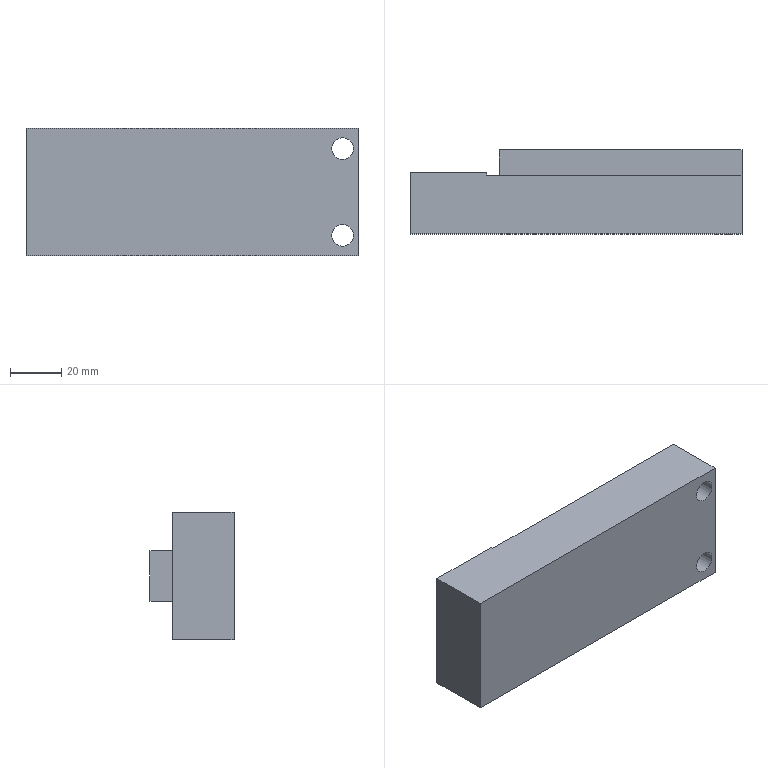Part | STEP file | SHIM SUPPORT | 1 solid | 18 faces | box 130 x 32.9 x 50 mm | volume 166423 mm3 | plane 12 | cylinder 4 | cone 2 | commonest cylinder face diameters 4.917 x2 8.5 x2
STEP:
#1=CARTESIAN_POINT('',(0.,0.,0.));
#2=DIRECTION('',(0.,0.,1.));
#3=DIRECTION('',(1.,0.,0.));
#4=AXIS2_PLACEMENT_3D('',#1,#2,#3);
#5=CARTESIAN_POINT('',(-103.5,89.682,-15.1));
#6=VERTEX_POINT('',#5);
#7=CARTESIAN_POINT('',(-103.5,79.782,-15.1));
#8=VERTEX_POINT('',#7);
#9=CARTESIAN_POINT('',(-103.5,89.682,-15.1));
#10=DIRECTION('',(0.,-1.,0.));
#11=VECTOR('',#10,1.);
#12=LINE('',#9,#11);
#13=CARTESIAN_POINT('',(-103.5,89.682,-34.9));
#14=DIRECTION('',(1.,0.,0.));
#15=DIRECTION('',(0.,0.,-1.));
#16=AXIS2_PLACEMENT_3D('',#13,#14,#15);
#17=PLANE('',#16);
#18=CARTESIAN_POINT('',(-19.8,0.));
#19=DIRECTION('',(0.,-1.));
#20=VECTOR('',#19,1.);
#21=LINE('',#18,#20);
#22=(GEOMETRIC_REPRESENTATION_CONTEXT(2)PARAMETRIC_REPRESENTATION_CONTEXT()REPRESENTATION_CONTEXT('',''));
#23=DEFINITIONAL_REPRESENTATION('',(#21),#22);
#24=PCURVE('',#17,#23);
#25=CARTESIAN_POINT('',(-108.5,79.782,-15.1));
#26=DIRECTION('',(0.,0.,1.));
#27=DIRECTION('',(1.,0.,0.));
#28=AXIS2_PLACEMENT_3D('',#25,#26,#27);
#29=PLANE('',#28);
#30=CARTESIAN_POINT('',(5.,9.9));
#31=DIRECTION('',(0.,-1.));
#32=VECTOR('',#31,1.);
#33=LINE('',#30,#32);
#34=(GEOMETRIC_REPRESENTATION_CONTEXT(2)PARAMETRIC_REPRESENTATION_CONTEXT()REPRESENTATION_CONTEXT('',''));
#35=DEFINITIONAL_REPRESENTATION('',(#33),#34);
#36=PCURVE('',#29,#35);
#37=SURFACE_CURVE('',#12,(#24,#36),.PCURVE_S1.);
#38=EDGE_CURVE('',#6,#8,#37,.T.);
#39=ORIENTED_EDGE('',*,*,#38,.F.);
#40=CARTESIAN_POINT('',(-103.5,89.682,-34.9));
#41=VERTEX_POINT('',#40);
#42=CARTESIAN_POINT('',(-103.5,89.682,-34.9));
#43=DIRECTION('',(0.,0.,1.));
#44=VECTOR('',#43,1.);
#45=LINE('',#42,#44);
#46=CARTESIAN_POINT('',(0.,0.));
#47=DIRECTION('',(-1.,0.));
#48=VECTOR('',#47,1.);
#49=LINE('',#46,#48);
#50=(GEOMETRIC_REPRESENTATION_CONTEXT(2)PARAMETRIC_REPRESENTATION_CONTEXT()REPRESENTATION_CONTEXT('',''));
#51=DEFINITIONAL_REPRESENTATION('',(#49),#50);
#52=PCURVE('',#17,#51);
#53=CARTESIAN_POINT('',(-108.5,89.682,-15.1));
#54=DIRECTION('',(0.,1.,0.));
#55=DIRECTION('',(0.,0.,1.));
#56=AXIS2_PLACEMENT_3D('',#53,#54,#55);
#57=PLANE('',#56);
#58=CARTESIAN_POINT('',(-19.8,5.));
#59=DIRECTION('',(1.,0.));
#60=VECTOR('',#59,1.);
#61=LINE('',#58,#60);
#62=(GEOMETRIC_REPRESENTATION_CONTEXT(2)PARAMETRIC_REPRESENTATION_CONTEXT()REPRESENTATION_CONTEXT('',''));
#63=DEFINITIONAL_REPRESENTATION('',(#61),#62);
#64=PCURVE('',#57,#63);
#65=SURFACE_CURVE('',#45,(#52,#64),.PCURVE_S1.);
#66=EDGE_CURVE('',#41,#6,#65,.T.);
#67=ORIENTED_EDGE('',*,*,#66,.F.);
#68=CARTESIAN_POINT('',(-103.5,79.782,-34.9));
#69=VERTEX_POINT('',#68);
#70=CARTESIAN_POINT('',(-103.5,79.782,-34.9));
#71=DIRECTION('',(0.,1.,0.));
#72=VECTOR('',#71,1.);
#73=LINE('',#70,#72);
#74=CARTESIAN_POINT('',(0.,-9.9));
#75=DIRECTION('',(0.,1.));
#76=VECTOR('',#75,1.);
#77=LINE('',#74,#76);
#78=(GEOMETRIC_REPRESENTATION_CONTEXT(2)PARAMETRIC_REPRESENTATION_CONTEXT()REPRESENTATION_CONTEXT('',''));
#79=DEFINITIONAL_REPRESENTATION('',(#77),#78);
#80=PCURVE('',#17,#79);
#81=CARTESIAN_POINT('',(-108.5,89.682,-34.9));
#82=DIRECTION('',(0.,0.,-1.));
#83=DIRECTION('',(-1.,0.,0.));
#84=AXIS2_PLACEMENT_3D('',#81,#82,#83);
#85=PLANE('',#84);
#86=CARTESIAN_POINT('',(-5.,-9.9));
#87=DIRECTION('',(0.,1.));
#88=VECTOR('',#87,1.);
#89=LINE('',#86,#88);
#90=(GEOMETRIC_REPRESENTATION_CONTEXT(2)PARAMETRIC_REPRESENTATION_CONTEXT()REPRESENTATION_CONTEXT('',''));
#91=DEFINITIONAL_REPRESENTATION('',(#89),#90);
#92=PCURVE('',#85,#91);
#93=SURFACE_CURVE('',#73,(#80,#92),.PCURVE_S1.);
#94=EDGE_CURVE('',#69,#41,#93,.T.);
#95=ORIENTED_EDGE('',*,*,#94,.F.);
#96=CARTESIAN_POINT('',(-103.5,79.782,-34.9));
#97=DIRECTION('',(0.,0.,1.));
#98=VECTOR('',#97,1.);
#99=LINE('',#96,#98);
#100=CARTESIAN_POINT('',(0.,-9.9));
#101=DIRECTION('',(-1.,0.));
#102=VECTOR('',#101,1.);
#103=LINE('',#100,#102);
#104=(GEOMETRIC_REPRESENTATION_CONTEXT(2)PARAMETRIC_REPRESENTATION_CONTEXT()REPRESENTATION_CONTEXT('',''));
#105=DEFINITIONAL_REPRESENTATION('',(#103),#104);
#106=PCURVE('',#17,#105);
#107=CARTESIAN_POINT('',(-8.5,79.782,0.));
#108=DIRECTION('',(0.,1.,0.));
#109=DIRECTION('',(0.,0.,1.));
#110=AXIS2_PLACEMENT_3D('',#107,#108,#109);
#111=PLANE('',#110);
#112=CARTESIAN_POINT('',(-34.9,-95.));
#113=DIRECTION('',(1.,0.));
#114=VECTOR('',#113,1.);
#115=LINE('',#112,#114);
#116=(GEOMETRIC_REPRESENTATION_CONTEXT(2)PARAMETRIC_REPRESENTATION_CONTEXT()REPRESENTATION_CONTEXT('',''));
#117=DEFINITIONAL_REPRESENTATION('',(#115),#116);
#118=PCURVE('',#111,#117);
#119=SURFACE_CURVE('',#99,(#106,#118),.PCURVE_S1.);
#120=EDGE_CURVE('',#69,#8,#119,.T.);
#121=ORIENTED_EDGE('',*,*,#120,.T.);
#122=EDGE_LOOP('',(#39,#67,#95,#121));
#123=FACE_BOUND('',#122,.T.);
#124=ADVANCED_FACE('',(#123),#17,.F.);
#125=ORIENTED_EDGE('',*,*,#94,.T.);
#126=CARTESIAN_POINT('',(-8.5,89.682,-34.9));
#127=VERTEX_POINT('',#126);
#128=CARTESIAN_POINT('',(-103.5,89.682,-34.9));
#129=DIRECTION('',(1.,0.,0.));
#130=VECTOR('',#129,1.);
#131=LINE('',#128,#130);
#132=CARTESIAN_POINT('',(-5.,0.));
#133=DIRECTION('',(-1.,0.));
#134=VECTOR('',#133,1.);
#135=LINE('',#132,#134);
#136=(GEOMETRIC_REPRESENTATION_CONTEXT(2)PARAMETRIC_REPRESENTATION_CONTEXT()REPRESENTATION_CONTEXT('',''));
#137=DEFINITIONAL_REPRESENTATION('',(#135),#136);
#138=PCURVE('',#85,#137);
#139=CARTESIAN_POINT('',(-19.8,5.));
#140=DIRECTION('',(0.,1.));
#141=VECTOR('',#140,1.);
#142=LINE('',#139,#141);
#143=(GEOMETRIC_REPRESENTATION_CONTEXT(2)PARAMETRIC_REPRESENTATION_CONTEXT()REPRESENTATION_CONTEXT('',''));
#144=DEFINITIONAL_REPRESENTATION('',(#142),#143);
#145=PCURVE('',#57,#144);
#146=SURFACE_CURVE('',#131,(#138,#145),.PCURVE_S1.);
#147=EDGE_CURVE('',#41,#127,#146,.T.);
#148=ORIENTED_EDGE('',*,*,#147,.T.);
#149=CARTESIAN_POINT('',(-8.5,79.782,-34.9));
#150=VERTEX_POINT('',#149);
#151=CARTESIAN_POINT('',(-8.5,89.682,-34.9));
#152=DIRECTION('',(0.,-1.,0.));
#153=VECTOR('',#152,1.);
#154=LINE('',#151,#153);
#155=CARTESIAN_POINT('',(-100.,0.));
#156=DIRECTION('',(0.,-1.));
#157=VECTOR('',#156,1.);
#158=LINE('',#155,#157);
#159=(GEOMETRIC_REPRESENTATION_CONTEXT(2)PARAMETRIC_REPRESENTATION_CONTEXT()REPRESENTATION_CONTEXT('',''));
#160=DEFINITIONAL_REPRESENTATION('',(#158),#159);
#161=PCURVE('',#85,#160);
#162=CARTESIAN_POINT('',(-8.5,56.782,0.));
#163=DIRECTION('',(1.,0.,0.));
#164=DIRECTION('',(0.,0.,-1.));
#165=AXIS2_PLACEMENT_3D('',#162,#163,#164);
#166=PLANE('',#165);
#167=CARTESIAN_POINT('',(34.9,32.9));
#168=DIRECTION('',(0.,-1.));
#169=VECTOR('',#168,1.);
#170=LINE('',#167,#169);
#171=(GEOMETRIC_REPRESENTATION_CONTEXT(2)PARAMETRIC_REPRESENTATION_CONTEXT()REPRESENTATION_CONTEXT('',''));
#172=DEFINITIONAL_REPRESENTATION('',(#170),#171);
#173=PCURVE('',#166,#172);
#174=SURFACE_CURVE('',#154,(#161,#173),.PCURVE_S1.);
#175=EDGE_CURVE('',#127,#150,#174,.T.);
#176=ORIENTED_EDGE('',*,*,#175,.T.);
#177=CARTESIAN_POINT('',(-103.5,79.782,-34.9));
#178=DIRECTION('',(1.,0.,0.));
#179=VECTOR('',#178,1.);
#180=LINE('',#177,#179);
#181=CARTESIAN_POINT('',(-5.,-9.9));
#182=DIRECTION('',(-1.,0.));
#183=VECTOR('',#182,1.);
#184=LINE('',#181,#183);
#185=(GEOMETRIC_REPRESENTATION_CONTEXT(2)PARAMETRIC_REPRESENTATION_CONTEXT()REPRESENTATION_CONTEXT('',''));
#186=DEFINITIONAL_REPRESENTATION('',(#184),#185);
#187=PCURVE('',#85,#186);
#188=CARTESIAN_POINT('',(-34.9,-95.));
#189=DIRECTION('',(0.,1.));
#190=VECTOR('',#189,1.);
#191=LINE('',#188,#190);
#192=(GEOMETRIC_REPRESENTATION_CONTEXT(2)PARAMETRIC_REPRESENTATION_CONTEXT()REPRESENTATION_CONTEXT('',''));
#193=DEFINITIONAL_REPRESENTATION('',(#191),#192);
#194=PCURVE('',#111,#193);
#195=SURFACE_CURVE('',#180,(#187,#194),.PCURVE_S1.);
#196=EDGE_CURVE('',#69,#150,#195,.T.);
#197=ORIENTED_EDGE('',*,*,#196,.F.);
#198=EDGE_LOOP('',(#125,#148,#176,#197));
#199=FACE_BOUND('',#198,.T.);
#200=ADVANCED_FACE('',(#199),#85,.T.);
#201=ORIENTED_EDGE('',*,*,#66,.T.);
#202=CARTESIAN_POINT('',(-8.5,89.682,-15.1));
#203=VERTEX_POINT('',#202);
#204=CARTESIAN_POINT('',(-103.5,89.682,-15.1));
#205=DIRECTION('',(1.,0.,0.));
#206=VECTOR('',#205,1.);
#207=LINE('',#204,#206);
#208=CARTESIAN_POINT('',(0.,5.));
#209=DIRECTION('',(0.,1.));
#210=VECTOR('',#209,1.);
#211=LINE('',#208,#210);
#212=(GEOMETRIC_REPRESENTATION_CONTEXT(2)PARAMETRIC_REPRESENTATION_CONTEXT()REPRESENTATION_CONTEXT('',''));
#213=DEFINITIONAL_REPRESENTATION('',(#211),#212);
#214=PCURVE('',#57,#213);
#215=CARTESIAN_POINT('',(5.,9.9));
#216=DIRECTION('',(1.,0.));
#217=VECTOR('',#216,1.);
#218=LINE('',#215,#217);
#219=(GEOMETRIC_REPRESENTATION_CONTEXT(2)PARAMETRIC_REPRESENTATION_CONTEXT()REPRESENTATION_CONTEXT('',''));
#220=DEFINITIONAL_REPRESENTATION('',(#218),#219);
#221=PCURVE('',#29,#220);
#222=SURFACE_CURVE('',#207,(#214,#221),.PCURVE_S1.);
#223=EDGE_CURVE('',#6,#203,#222,.T.);
#224=ORIENTED_EDGE('',*,*,#223,.T.);
#225=CARTESIAN_POINT('',(-8.5,89.682,-15.1));
#226=DIRECTION('',(0.,0.,-1.));
#227=VECTOR('',#226,1.);
#228=LINE('',#225,#227);
#229=CARTESIAN_POINT('',(0.,100.));
#230=DIRECTION('',(-1.,0.));
#231=VECTOR('',#230,1.);
#232=LINE('',#229,#231);
#233=(GEOMETRIC_REPRESENTATION_CONTEXT(2)PARAMETRIC_REPRESENTATION_CONTEXT()REPRESENTATION_CONTEXT('',''));
#234=DEFINITIONAL_REPRESENTATION('',(#232),#233);
#235=PCURVE('',#57,#234);
#236=CARTESIAN_POINT('',(15.1,32.9));
#237=DIRECTION('',(1.,0.));
#238=VECTOR('',#237,1.);
#239=LINE('',#236,#238);
#240=(GEOMETRIC_REPRESENTATION_CONTEXT(2)PARAMETRIC_REPRESENTATION_CONTEXT()REPRESENTATION_CONTEXT('',''));
#241=DEFINITIONAL_REPRESENTATION('',(#239),#240);
#242=PCURVE('',#166,#241);
#243=SURFACE_CURVE('',#228,(#235,#242),.PCURVE_S1.);
#244=EDGE_CURVE('',#203,#127,#243,.T.);
#245=ORIENTED_EDGE('',*,*,#244,.T.);
#246=ORIENTED_EDGE('',*,*,#147,.F.);
#247=EDGE_LOOP('',(#201,#224,#245,#246));
#248=FACE_BOUND('',#247,.T.);
#249=ADVANCED_FACE('',(#248),#57,.T.);
#250=CARTESIAN_POINT('',(-114.775,65.782,-5.));
#251=VERTEX_POINT('',#250);
#252=CARTESIAN_POINT('',(-117.233,65.782,-5.));
#253=DIRECTION('',(0.,1.,0.));
#254=DIRECTION('',(1.,0.,0.));
#255=AXIS2_PLACEMENT_3D('',#252,#253,#254);
#256=CIRCLE('',#255,2.458);
#257=CARTESIAN_POINT('',(-117.233,65.043,-5.));
#258=DIRECTION('',(0.,1.,0.));
#259=DIRECTION('',(1.,0.,0.));
#260=AXIS2_PLACEMENT_3D('',#257,#258,#259);
#261=CONICAL_SURFACE('',#260,1.229,1.03);
#262=CARTESIAN_POINT('',(0.,0.7386));
#263=DIRECTION('',(1.,0.));
#264=VECTOR('',#263,1.);
#265=LINE('',#262,#264);
#266=(GEOMETRIC_REPRESENTATION_CONTEXT(2)PARAMETRIC_REPRESENTATION_CONTEXT()REPRESENTATION_CONTEXT('',''));
#267=DEFINITIONAL_REPRESENTATION('',(#265),#266);
#268=PCURVE('',#261,#267);
#269=CARTESIAN_POINT('',(-117.233,73.282,-5.));
#270=DIRECTION('',(0.,1.,0.));
#271=DIRECTION('',(1.,0.,0.));
#272=AXIS2_PLACEMENT_3D('',#269,#270,#271);
#273=CYLINDRICAL_SURFACE('',#272,2.458);
#274=CARTESIAN_POINT('',(0.,-7.5));
#275=DIRECTION('',(1.,0.));
#276=VECTOR('',#275,1.);
#277=LINE('',#274,#276);
#278=(GEOMETRIC_REPRESENTATION_CONTEXT(2)PARAMETRIC_REPRESENTATION_CONTEXT()REPRESENTATION_CONTEXT('',''));
#279=DEFINITIONAL_REPRESENTATION('',(#277),#278);
#280=PCURVE('',#273,#279);
#281=SURFACE_CURVE('',#256,(#268,#280),.PCURVE_S1.);
#282=EDGE_CURVE('',#251,#251,#281,.T.);
#283=ORIENTED_EDGE('',*,*,#282,.F.);
#284=CARTESIAN_POINT('',(-117.233,64.304,-5.));
#285=VERTEX_POINT('',#284);
#286=CARTESIAN_POINT('',(-117.233,64.304,-5.));
#287=CARTESIAN_POINT('',(-114.775,65.782,-5.));
#288=B_SPLINE_CURVE_WITH_KNOTS('',1,(#286,#287),.UNSPECIFIED.,.F.,.F.,(2,2),(-1.434,1.434),.PIECEWISE_BEZIER_KNOTS.);
#289=CARTESIAN_POINT('',(0.,0.));
#290=DIRECTION('',(0.,1.));
#291=VECTOR('',#290,1.);
#292=LINE('',#289,#291);
#293=(GEOMETRIC_REPRESENTATION_CONTEXT(2)PARAMETRIC_REPRESENTATION_CONTEXT()REPRESENTATION_CONTEXT('',''));
#294=DEFINITIONAL_REPRESENTATION('',(#292),#293);
#295=PCURVE('',#261,#294);
#296=CARTESIAN_POINT('',(6.283,0.));
#297=DIRECTION('',(0.,1.));
#298=VECTOR('',#297,1.);
#299=LINE('',#296,#298);
#300=(GEOMETRIC_REPRESENTATION_CONTEXT(2)PARAMETRIC_REPRESENTATION_CONTEXT()REPRESENTATION_CONTEXT('',''));
#301=DEFINITIONAL_REPRESENTATION('',(#299),#300);
#302=PCURVE('',#261,#301);
#303=SEAM_CURVE('',#288,(#295,#302),.PCURVE_S1.);
#304=EDGE_CURVE('',#285,#251,#303,.T.);
#305=ORIENTED_EDGE('',*,*,#304,.F.);
#306=ORIENTED_EDGE('',*,*,#304,.T.);
#307=EDGE_LOOP('',(#283,#305,#306));
#308=FACE_BOUND('',#307,.F.);
#309=ADVANCED_FACE('',(#308),#261,.F.);
#310=CARTESIAN_POINT('',(-114.775,80.782,-5.));
#311=VERTEX_POINT('',#310);
#312=CARTESIAN_POINT('',(-117.233,80.782,-5.));
#313=DIRECTION('',(0.,-1.,0.));
#314=DIRECTION('',(1.,0.,0.));
#315=AXIS2_PLACEMENT_3D('',#312,#313,#314);
#316=CIRCLE('',#315,2.458);
#317=CARTESIAN_POINT('',(6.283,7.5));
#318=DIRECTION('',(-1.,0.));
#319=VECTOR('',#318,1.);
#320=LINE('',#317,#319);
#321=(GEOMETRIC_REPRESENTATION_CONTEXT(2)PARAMETRIC_REPRESENTATION_CONTEXT()REPRESENTATION_CONTEXT('',''));
#322=DEFINITIONAL_REPRESENTATION('',(#320),#321);
#323=PCURVE('',#273,#322);
#324=CARTESIAN_POINT('',(-108.5,80.782,-50.));
#325=DIRECTION('',(0.,1.,0.));
#326=DIRECTION('',(0.,0.,1.));
#327=AXIS2_PLACEMENT_3D('',#324,#325,#326);
#328=PLANE('',#327);
#329=CARTESIAN_POINT('',(45.,-6.275));
#330=CARTESIAN_POINT('',(49.258,-6.275));
#331=CARTESIAN_POINT('',(47.129,-9.962));
#332=CARTESIAN_POINT('',(45.,-13.65));
#333=CARTESIAN_POINT('',(42.871,-9.962));
#334=CARTESIAN_POINT('',(40.742,-6.275));
#335=CARTESIAN_POINT('',(45.,-6.275));
#336=(BOUNDED_CURVE()B_SPLINE_CURVE(2,(#329,#330,#331,#332,#333,#334,#335),.UNSPECIFIED.,.T.,.F.)B_SPLINE_CURVE_WITH_KNOTS((1,2,2,2,2,1),(-2.094,0.,2.094,4.189,6.283,8.378),.UNSPECIFIED.)CURVE()GEOMETRIC_REPRESENTATION_ITEM()RATIONAL_B_SPLINE_CURVE((1.,0.5,1.,0.5,1.,0.5,1.))REPRESENTATION_ITEM(''));
#337=(GEOMETRIC_REPRESENTATION_CONTEXT(2)PARAMETRIC_REPRESENTATION_CONTEXT()REPRESENTATION_CONTEXT('',''));
#338=DEFINITIONAL_REPRESENTATION('',(#336),#337);
#339=PCURVE('',#328,#338);
#340=SURFACE_CURVE('',#316,(#323,#339),.PCURVE_S1.);
#341=EDGE_CURVE('',#311,#311,#340,.T.);
#342=ORIENTED_EDGE('',*,*,#341,.T.);
#343=CARTESIAN_POINT('',(-114.775,65.782,-5.));
#344=CARTESIAN_POINT('',(-114.775,80.782,-5.));
#345=B_SPLINE_CURVE_WITH_KNOTS('',1,(#343,#344),.UNSPECIFIED.,.F.,.F.,(2,2),(-7.5,7.5),.PIECEWISE_BEZIER_KNOTS.);
#346=CARTESIAN_POINT('',(0.,0.));
#347=DIRECTION('',(0.,1.));
#348=VECTOR('',#347,1.);
#349=LINE('',#346,#348);
#350=(GEOMETRIC_REPRESENTATION_CONTEXT(2)PARAMETRIC_REPRESENTATION_CONTEXT()REPRESENTATION_CONTEXT('',''));
#351=DEFINITIONAL_REPRESENTATION('',(#349),#350);
#352=PCURVE('',#273,#351);
#353=CARTESIAN_POINT('',(6.283,0.));
#354=DIRECTION('',(0.,1.));
#355=VECTOR('',#354,1.);
#356=LINE('',#353,#355);
#357=(GEOMETRIC_REPRESENTATION_CONTEXT(2)PARAMETRIC_REPRESENTATION_CONTEXT()REPRESENTATION_CONTEXT('',''));
#358=DEFINITIONAL_REPRESENTATION('',(#356),#357);
#359=PCURVE('',#273,#358);
#360=SEAM_CURVE('',#345,(#352,#359),.PCURVE_S1.);
#361=EDGE_CURVE('',#251,#311,#360,.T.);
#362=ORIENTED_EDGE('',*,*,#361,.F.);
#363=ORIENTED_EDGE('',*,*,#282,.T.);
#364=ORIENTED_EDGE('',*,*,#361,.T.);
#365=EDGE_LOOP('',(#342,#362,#363,#364));
#366=FACE_BOUND('',#365,.F.);
#367=ADVANCED_FACE('',(#366),#273,.F.);
#368=CARTESIAN_POINT('',(-114.775,65.782,-45.));
#369=VERTEX_POINT('',#368);
#370=CARTESIAN_POINT('',(-117.233,65.782,-45.));
#371=DIRECTION('',(0.,1.,0.));
#372=DIRECTION('',(1.,0.,0.));
#373=AXIS2_PLACEMENT_3D('',#370,#371,#372);
#374=CIRCLE('',#373,2.458);
#375=CARTESIAN_POINT('',(-117.233,65.043,-45.));
#376=DIRECTION('',(0.,1.,0.));
#377=DIRECTION('',(1.,0.,0.));
#378=AXIS2_PLACEMENT_3D('',#375,#376,#377);
#379=CONICAL_SURFACE('',#378,1.229,1.03);
#380=CARTESIAN_POINT('',(0.,0.7386));
#381=DIRECTION('',(1.,0.));
#382=VECTOR('',#381,1.);
#383=LINE('',#380,#382);
#384=(GEOMETRIC_REPRESENTATION_CONTEXT(2)PARAMETRIC_REPRESENTATION_CONTEXT()REPRESENTATION_CONTEXT('',''));
#385=DEFINITIONAL_REPRESENTATION('',(#383),#384);
#386=PCURVE('',#379,#385);
#387=CARTESIAN_POINT('',(-117.233,73.282,-45.));
#388=DIRECTION('',(0.,1.,0.));
#389=DIRECTION('',(1.,0.,0.));
#390=AXIS2_PLACEMENT_3D('',#387,#388,#389);
#391=CYLINDRICAL_SURFACE('',#390,2.458);
#392=CARTESIAN_POINT('',(0.,-7.5));
#393=DIRECTION('',(1.,0.));
#394=VECTOR('',#393,1.);
#395=LINE('',#392,#394);
#396=(GEOMETRIC_REPRESENTATION_CONTEXT(2)PARAMETRIC_REPRESENTATION_CONTEXT()REPRESENTATION_CONTEXT('',''));
#397=DEFINITIONAL_REPRESENTATION('',(#395),#396);
#398=PCURVE('',#391,#397);
#399=SURFACE_CURVE('',#374,(#386,#398),.PCURVE_S1.);
#400=EDGE_CURVE('',#369,#369,#399,.T.);
#401=ORIENTED_EDGE('',*,*,#400,.F.);
#402=CARTESIAN_POINT('',(-117.233,64.304,-45.));
#403=VERTEX_POINT('',#402);
#404=CARTESIAN_POINT('',(-117.233,64.304,-45.));
#405=CARTESIAN_POINT('',(-114.775,65.782,-45.));
#406=B_SPLINE_CURVE_WITH_KNOTS('',1,(#404,#405),.UNSPECIFIED.,.F.,.F.,(2,2),(-1.434,1.434),.PIECEWISE_BEZIER_KNOTS.);
#407=CARTESIAN_POINT('',(0.,0.));
#408=DIRECTION('',(0.,1.));
#409=VECTOR('',#408,1.);
#410=LINE('',#407,#409);
#411=(GEOMETRIC_REPRESENTATION_CONTEXT(2)PARAMETRIC_REPRESENTATION_CONTEXT()REPRESENTATION_CONTEXT('',''));
#412=DEFINITIONAL_REPRESENTATION('',(#410),#411);
#413=PCURVE('',#379,#412);
#414=CARTESIAN_POINT('',(6.283,0.));
#415=DIRECTION('',(0.,1.));
#416=VECTOR('',#415,1.);
#417=LINE('',#414,#416);
#418=(GEOMETRIC_REPRESENTATION_CONTEXT(2)PARAMETRIC_REPRESENTATION_CONTEXT()REPRESENTATION_CONTEXT('',''));
#419=DEFINITIONAL_REPRESENTATION('',(#417),#418);
#420=PCURVE('',#379,#419);
#421=SEAM_CURVE('',#406,(#413,#420),.PCURVE_S1.);
#422=EDGE_CURVE('',#403,#369,#421,.T.);
#423=ORIENTED_EDGE('',*,*,#422,.F.);
#424=ORIENTED_EDGE('',*,*,#422,.T.);
#425=EDGE_LOOP('',(#401,#423,#424));
#426=FACE_BOUND('',#425,.F.);
#427=ADVANCED_FACE('',(#426),#379,.F.);
#428=CARTESIAN_POINT('',(-114.775,80.782,-45.));
#429=VERTEX_POINT('',#428);
#430=CARTESIAN_POINT('',(-117.233,80.782,-45.));
#431=DIRECTION('',(0.,-1.,0.));
#432=DIRECTION('',(1.,0.,0.));
#433=AXIS2_PLACEMENT_3D('',#430,#431,#432);
#434=CIRCLE('',#433,2.458);
#435=CARTESIAN_POINT('',(6.283,7.5));
#436=DIRECTION('',(-1.,0.));
#437=VECTOR('',#436,1.);
#438=LINE('',#435,#437);
#439=(GEOMETRIC_REPRESENTATION_CONTEXT(2)PARAMETRIC_REPRESENTATION_CONTEXT()REPRESENTATION_CONTEXT('',''));
#440=DEFINITIONAL_REPRESENTATION('',(#438),#439);
#441=PCURVE('',#391,#440);
#442=CARTESIAN_POINT('',(5.,-6.275));
#443=CARTESIAN_POINT('',(9.258,-6.275));
#444=CARTESIAN_POINT('',(7.129,-9.962));
#445=CARTESIAN_POINT('',(5.,-13.65));
#446=CARTESIAN_POINT('',(2.871,-9.962));
#447=CARTESIAN_POINT('',(0.7418,-6.275));
#448=CARTESIAN_POINT('',(5.,-6.275));
#449=(BOUNDED_CURVE()B_SPLINE_CURVE(2,(#442,#443,#444,#445,#446,#447,#448),.UNSPECIFIED.,.T.,.F.)B_SPLINE_CURVE_WITH_KNOTS((1,2,2,2,2,1),(-2.094,0.,2.094,4.189,6.283,8.378),.UNSPECIFIED.)CURVE()GEOMETRIC_REPRESENTATION_ITEM()RATIONAL_B_SPLINE_CURVE((1.,0.5,1.,0.5,1.,0.5,1.))REPRESENTATION_ITEM(''));
#450=(GEOMETRIC_REPRESENTATION_CONTEXT(2)PARAMETRIC_REPRESENTATION_CONTEXT()REPRESENTATION_CONTEXT('',''));
#451=DEFINITIONAL_REPRESENTATION('',(#449),#450);
#452=PCURVE('',#328,#451);
#453=SURFACE_CURVE('',#434,(#441,#452),.PCURVE_S1.);
#454=EDGE_CURVE('',#429,#429,#453,.T.);
#455=ORIENTED_EDGE('',*,*,#454,.T.);
#456=CARTESIAN_POINT('',(-114.775,65.782,-45.));
#457=CARTESIAN_POINT('',(-114.775,80.782,-45.));
#458=B_SPLINE_CURVE_WITH_KNOTS('',1,(#456,#457),.UNSPECIFIED.,.F.,.F.,(2,2),(-7.5,7.5),.PIECEWISE_BEZIER_KNOTS.);
#459=CARTESIAN_POINT('',(0.,0.));
#460=DIRECTION('',(0.,1.));
#461=VECTOR('',#460,1.);
#462=LINE('',#459,#461);
#463=(GEOMETRIC_REPRESENTATION_CONTEXT(2)PARAMETRIC_REPRESENTATION_CONTEXT()REPRESENTATION_CONTEXT('',''));
#464=DEFINITIONAL_REPRESENTATION('',(#462),#463);
#465=PCURVE('',#391,#464);
#466=CARTESIAN_POINT('',(6.283,0.));
#467=DIRECTION('',(0.,1.));
#468=VECTOR('',#467,1.);
#469=LINE('',#466,#468);
#470=(GEOMETRIC_REPRESENTATION_CONTEXT(2)PARAMETRIC_REPRESENTATION_CONTEXT()REPRESENTATION_CONTEXT('',''));
#471=DEFINITIONAL_REPRESENTATION('',(#469),#470);
#472=PCURVE('',#391,#471);
#473=SEAM_CURVE('',#458,(#465,#472),.PCURVE_S1.);
#474=EDGE_CURVE('',#369,#429,#473,.T.);
#475=ORIENTED_EDGE('',*,*,#474,.F.);
#476=ORIENTED_EDGE('',*,*,#400,.T.);
#477=ORIENTED_EDGE('',*,*,#474,.T.);
#478=EDGE_LOOP('',(#455,#475,#476,#477));
#479=FACE_BOUND('',#478,.F.);
#480=ADVANCED_FACE('',(#479),#391,.F.);
#481=CARTESIAN_POINT('',(-18.75,56.782,-42.));
#482=VERTEX_POINT('',#481);
#483=CARTESIAN_POINT('',(-10.25,56.782,-42.));
#484=VERTEX_POINT('',#483);
#485=CARTESIAN_POINT('',(-14.5,56.782,-42.));
#486=DIRECTION('',(0.,1.,0.));
#487=DIRECTION('',(1.,0.,0.));
#488=AXIS2_PLACEMENT_3D('',#485,#486,#487);
#489=CIRCLE('',#488,4.25);
#490=CARTESIAN_POINT('',(-14.5,-63.335,-42.));
#491=DIRECTION('',(0.,1.,0.));
#492=DIRECTION('',(1.,0.,0.));
#493=AXIS2_PLACEMENT_3D('',#490,#491,#492);
#494=CYLINDRICAL_SURFACE('',#493,4.25);
#495=CARTESIAN_POINT('',(0.,120.117));
#496=DIRECTION('',(1.,0.));
#497=VECTOR('',#496,1.);
#498=LINE('',#495,#497);
#499=(GEOMETRIC_REPRESENTATION_CONTEXT(2)PARAMETRIC_REPRESENTATION_CONTEXT()REPRESENTATION_CONTEXT('',''));
#500=DEFINITIONAL_REPRESENTATION('',(#498),#499);
#501=PCURVE('',#494,#500);
#502=CARTESIAN_POINT('',(-18.5,56.782,0.));
#503=DIRECTION('',(0.,-1.,0.));
#504=DIRECTION('',(0.,0.,-1.));
#505=AXIS2_PLACEMENT_3D('',#502,#503,#504);
#506=PLANE('',#505);
#507=CARTESIAN_POINT('',(42.,8.25));
#508=CARTESIAN_POINT('',(49.361,8.25));
#509=CARTESIAN_POINT('',(45.681,1.875));
#510=CARTESIAN_POINT('',(42.,-4.5));
#511=CARTESIAN_POINT('',(38.319,1.875));
#512=CARTESIAN_POINT('',(34.639,8.25));
#513=CARTESIAN_POINT('',(42.,8.25));
#514=(BOUNDED_CURVE()B_SPLINE_CURVE(2,(#507,#508,#509,#510,#511,#512,#513),.UNSPECIFIED.,.T.,.F.)B_SPLINE_CURVE_WITH_KNOTS((1,2,2,2,2,1),(-2.094,0.,2.094,4.189,6.283,8.378),.UNSPECIFIED.)CURVE()GEOMETRIC_REPRESENTATION_ITEM()RATIONAL_B_SPLINE_CURVE((1.,0.5,1.,0.5,1.,0.5,1.))REPRESENTATION_ITEM(''));
#515=(GEOMETRIC_REPRESENTATION_CONTEXT(2)PARAMETRIC_REPRESENTATION_CONTEXT()REPRESENTATION_CONTEXT('',''));
#516=DEFINITIONAL_REPRESENTATION('',(#514),#515);
#517=PCURVE('',#506,#516);
#518=SURFACE_CURVE('',#489,(#501,#517),.PCURVE_S1.);
#519=EDGE_CURVE('',#482,#484,#518,.T.);
#520=ORIENTED_EDGE('',*,*,#519,.T.);
#521=CARTESIAN_POINT('',(-10.25,79.782,-42.));
#522=VERTEX_POINT('',#521);
#523=CARTESIAN_POINT('',(-10.25,56.782,-42.));
#524=CARTESIAN_POINT('',(-10.25,79.782,-42.));
#525=B_SPLINE_CURVE_WITH_KNOTS('',1,(#523,#524),.UNSPECIFIED.,.F.,.F.,(2,2),(120.117,143.117),.PIECEWISE_BEZIER_KNOTS.);
#526=CARTESIAN_POINT('',(6.283,0.));
#527=DIRECTION('',(0.,1.));
#528=VECTOR('',#527,1.);
#529=LINE('',#526,#528);
#530=(GEOMETRIC_REPRESENTATION_CONTEXT(2)PARAMETRIC_REPRESENTATION_CONTEXT()REPRESENTATION_CONTEXT('',''));
#531=DEFINITIONAL_REPRESENTATION('',(#529),#530);
#532=PCURVE('',#494,#531);
#533=CARTESIAN_POINT('',(0.,0.));
#534=DIRECTION('',(0.,1.));
#535=VECTOR('',#534,1.);
#536=LINE('',#533,#535);
#537=(GEOMETRIC_REPRESENTATION_CONTEXT(2)PARAMETRIC_REPRESENTATION_CONTEXT()REPRESENTATION_CONTEXT('',''));
#538=DEFINITIONAL_REPRESENTATION('',(#536),#537);
#539=PCURVE('',#494,#538);
#540=SEAM_CURVE('',#525,(#532,#539),.PCURVE_S1.);
#541=EDGE_CURVE('',#484,#522,#540,.T.);
#542=ORIENTED_EDGE('',*,*,#541,.T.);
#543=CARTESIAN_POINT('',(-14.5,79.782,-42.));
#544=DIRECTION('',(0.,-1.,0.));
#545=DIRECTION('',(1.,0.,0.));
#546=AXIS2_PLACEMENT_3D('',#543,#544,#545);
#547=CIRCLE('',#546,4.25);
#548=CARTESIAN_POINT('',(6.283,143.117));
#549=DIRECTION('',(-1.,0.));
#550=VECTOR('',#549,1.);
#551=LINE('',#548,#550);
#552=(GEOMETRIC_REPRESENTATION_CONTEXT(2)PARAMETRIC_REPRESENTATION_CONTEXT()REPRESENTATION_CONTEXT('',''));
#553=DEFINITIONAL_REPRESENTATION('',(#551),#552);
#554=PCURVE('',#494,#553);
#555=CARTESIAN_POINT('',(-42.,-1.75));
#556=CARTESIAN_POINT('',(-34.639,-1.75));
#557=CARTESIAN_POINT('',(-38.319,-8.125));
#558=CARTESIAN_POINT('',(-42.,-14.5));
#559=CARTESIAN_POINT('',(-45.681,-8.125));
#560=CARTESIAN_POINT('',(-49.361,-1.75));
#561=CARTESIAN_POINT('',(-42.,-1.75));
#562=(BOUNDED_CURVE()B_SPLINE_CURVE(2,(#555,#556,#557,#558,#559,#560,#561),.UNSPECIFIED.,.T.,.F.)B_SPLINE_CURVE_WITH_KNOTS((1,2,2,2,2,1),(-2.094,0.,2.094,4.189,6.283,8.378),.UNSPECIFIED.)CURVE()GEOMETRIC_REPRESENTATION_ITEM()RATIONAL_B_SPLINE_CURVE((1.,0.5,1.,0.5,1.,0.5,1.))REPRESENTATION_ITEM(''));
#563=(GEOMETRIC_REPRESENTATION_CONTEXT(2)PARAMETRIC_REPRESENTATION_CONTEXT()REPRESENTATION_CONTEXT('',''));
#564=DEFINITIONAL_REPRESENTATION('',(#562),#563);
#565=PCURVE('',#111,#564);
#566=SURFACE_CURVE('',#547,(#554,#565),.PCURVE_S1.);
#567=EDGE_CURVE('',#522,#522,#566,.T.);
#568=ORIENTED_EDGE('',*,*,#567,.T.);
#569=ORIENTED_EDGE('',*,*,#541,.F.);
#570=CARTESIAN_POINT('',(-14.5,56.782,-42.));
#571=DIRECTION('',(0.,1.,0.));
#572=DIRECTION('',(1.,0.,0.));
#573=AXIS2_PLACEMENT_3D('',#570,#571,#572);
#574=CIRCLE('',#573,4.25);
#575=CARTESIAN_POINT('',(-6.283,120.117));
#576=DIRECTION('',(1.,0.));
#577=VECTOR('',#576,1.);
#578=LINE('',#575,#577);
#579=(GEOMETRIC_REPRESENTATION_CONTEXT(2)PARAMETRIC_REPRESENTATION_CONTEXT()REPRESENTATION_CONTEXT('',''));
#580=DEFINITIONAL_REPRESENTATION('',(#578),#579);
#581=PCURVE('',#494,#580);
#582=CARTESIAN_POINT('',(42.,8.25));
#583=CARTESIAN_POINT('',(49.361,8.25));
#584=CARTESIAN_POINT('',(45.681,1.875));
#585=CARTESIAN_POINT('',(42.,-4.5));
#586=CARTESIAN_POINT('',(38.319,1.875));
#587=CARTESIAN_POINT('',(34.639,8.25));
#588=CARTESIAN_POINT('',(42.,8.25));
#589=(BOUNDED_CURVE()B_SPLINE_CURVE(2,(#582,#583,#584,#585,#586,#587,#588),.UNSPECIFIED.,.T.,.F.)B_SPLINE_CURVE_WITH_KNOTS((1,2,2,2,2,1),(-2.094,0.,2.094,4.189,6.283,8.378),.UNSPECIFIED.)CURVE()GEOMETRIC_REPRESENTATION_ITEM()RATIONAL_B_SPLINE_CURVE((1.,0.5,1.,0.5,1.,0.5,1.))REPRESENTATION_ITEM(''));
#590=(GEOMETRIC_REPRESENTATION_CONTEXT(2)PARAMETRIC_REPRESENTATION_CONTEXT()REPRESENTATION_CONTEXT('',''));
#591=DEFINITIONAL_REPRESENTATION('',(#589),#590);
#592=PCURVE('',#506,#591);
#593=SURFACE_CURVE('',#574,(#581,#592),.PCURVE_S1.);
#594=EDGE_CURVE('',#484,#482,#593,.T.);
#595=ORIENTED_EDGE('',*,*,#594,.T.);
#596=EDGE_LOOP('',(#520,#542,#568,#569,#595));
#597=FACE_BOUND('',#596,.F.);
#598=ADVANCED_FACE('',(#597),#494,.F.);
#599=CARTESIAN_POINT('',(-18.75,56.782,-8.));
#600=VERTEX_POINT('',#599);
#601=CARTESIAN_POINT('',(-10.25,56.782,-8.));
#602=VERTEX_POINT('',#601);
#603=CARTESIAN_POINT('',(-14.5,56.782,-8.));
#604=DIRECTION('',(0.,1.,0.));
#605=DIRECTION('',(1.,0.,0.));
#606=AXIS2_PLACEMENT_3D('',#603,#604,#605);
#607=CIRCLE('',#606,4.25);
#608=CARTESIAN_POINT('',(-14.5,-63.335,-8.));
#609=DIRECTION('',(0.,1.,0.));
#610=DIRECTION('',(1.,0.,0.));
#611=AXIS2_PLACEMENT_3D('',#608,#609,#610);
#612=CYLINDRICAL_SURFACE('',#611,4.25);
#613=CARTESIAN_POINT('',(0.,120.117));
#614=DIRECTION('',(1.,0.));
#615=VECTOR('',#614,1.);
#616=LINE('',#613,#615);
#617=(GEOMETRIC_REPRESENTATION_CONTEXT(2)PARAMETRIC_REPRESENTATION_CONTEXT()REPRESENTATION_CONTEXT('',''));
#618=DEFINITIONAL_REPRESENTATION('',(#616),#617);
#619=PCURVE('',#612,#618);
#620=CARTESIAN_POINT('',(8.,8.25));
#621=CARTESIAN_POINT('',(15.361,8.25));
#622=CARTESIAN_POINT('',(11.681,1.875));
#623=CARTESIAN_POINT('',(8.,-4.5));
#624=CARTESIAN_POINT('',(4.319,1.875));
#625=CARTESIAN_POINT('',(0.6388,8.25));
#626=CARTESIAN_POINT('',(8.,8.25));
#627=(BOUNDED_CURVE()B_SPLINE_CURVE(2,(#620,#621,#622,#623,#624,#625,#626),.UNSPECIFIED.,.T.,.F.)B_SPLINE_CURVE_WITH_KNOTS((1,2,2,2,2,1),(-2.094,0.,2.094,4.189,6.283,8.378),.UNSPECIFIED.)CURVE()GEOMETRIC_REPRESENTATION_ITEM()RATIONAL_B_SPLINE_CURVE((1.,0.5,1.,0.5,1.,0.5,1.))REPRESENTATION_ITEM(''));
#628=(GEOMETRIC_REPRESENTATION_CONTEXT(2)PARAMETRIC_REPRESENTATION_CONTEXT()REPRESENTATION_CONTEXT('',''));
#629=DEFINITIONAL_REPRESENTATION('',(#627),#628);
#630=PCURVE('',#506,#629);
#631=SURFACE_CURVE('',#607,(#619,#630),.PCURVE_S1.);
#632=EDGE_CURVE('',#600,#602,#631,.T.);
#633=ORIENTED_EDGE('',*,*,#632,.T.);
#634=CARTESIAN_POINT('',(-10.25,79.782,-8.));
#635=VERTEX_POINT('',#634);
#636=CARTESIAN_POINT('',(-10.25,56.782,-8.));
#637=CARTESIAN_POINT('',(-10.25,79.782,-8.));
#638=B_SPLINE_CURVE_WITH_KNOTS('',1,(#636,#637),.UNSPECIFIED.,.F.,.F.,(2,2),(120.117,143.117),.PIECEWISE_BEZIER_KNOTS.);
#639=CARTESIAN_POINT('',(6.283,0.));
#640=DIRECTION('',(0.,1.));
#641=VECTOR('',#640,1.);
#642=LINE('',#639,#641);
#643=(GEOMETRIC_REPRESENTATION_CONTEXT(2)PARAMETRIC_REPRESENTATION_CONTEXT()REPRESENTATION_CONTEXT('',''));
#644=DEFINITIONAL_REPRESENTATION('',(#642),#643);
#645=PCURVE('',#612,#644);
#646=CARTESIAN_POINT('',(0.,0.));
#647=DIRECTION('',(0.,1.));
#648=VECTOR('',#647,1.);
#649=LINE('',#646,#648);
#650=(GEOMETRIC_REPRESENTATION_CONTEXT(2)PARAMETRIC_REPRESENTATION_CONTEXT()REPRESENTATION_CONTEXT('',''));
#651=DEFINITIONAL_REPRESENTATION('',(#649),#650);
#652=PCURVE('',#612,#651);
#653=SEAM_CURVE('',#638,(#645,#652),.PCURVE_S1.);
#654=EDGE_CURVE('',#602,#635,#653,.T.);
#655=ORIENTED_EDGE('',*,*,#654,.T.);
#656=CARTESIAN_POINT('',(-14.5,79.782,-8.));
#657=DIRECTION('',(0.,-1.,0.));
#658=DIRECTION('',(1.,0.,0.));
#659=AXIS2_PLACEMENT_3D('',#656,#657,#658);
#660=CIRCLE('',#659,4.25);
#661=CARTESIAN_POINT('',(6.283,143.117));
#662=DIRECTION('',(-1.,0.));
#663=VECTOR('',#662,1.);
#664=LINE('',#661,#663);
#665=(GEOMETRIC_REPRESENTATION_CONTEXT(2)PARAMETRIC_REPRESENTATION_CONTEXT()REPRESENTATION_CONTEXT('',''));
#666=DEFINITIONAL_REPRESENTATION('',(#664),#665);
#667=PCURVE('',#612,#666);
#668=CARTESIAN_POINT('',(-8.,-1.75));
#669=CARTESIAN_POINT('',(-0.6388,-1.75));
#670=CARTESIAN_POINT('',(-4.319,-8.125));
#671=CARTESIAN_POINT('',(-8.,-14.5));
#672=CARTESIAN_POINT('',(-11.681,-8.125));
#673=CARTESIAN_POINT('',(-15.361,-1.75));
#674=CARTESIAN_POINT('',(-8.,-1.75));
#675=(BOUNDED_CURVE()B_SPLINE_CURVE(2,(#668,#669,#670,#671,#672,#673,#674),.UNSPECIFIED.,.T.,.F.)B_SPLINE_CURVE_WITH_KNOTS((1,2,2,2,2,1),(-2.094,0.,2.094,4.189,6.283,8.378),.UNSPECIFIED.)CURVE()GEOMETRIC_REPRESENTATION_ITEM()RATIONAL_B_SPLINE_CURVE((1.,0.5,1.,0.5,1.,0.5,1.))REPRESENTATION_ITEM(''));
#676=(GEOMETRIC_REPRESENTATION_CONTEXT(2)PARAMETRIC_REPRESENTATION_CONTEXT()REPRESENTATION_CONTEXT('',''));
#677=DEFINITIONAL_REPRESENTATION('',(#675),#676);
#678=PCURVE('',#111,#677);
#679=SURFACE_CURVE('',#660,(#667,#678),.PCURVE_S1.);
#680=EDGE_CURVE('',#635,#635,#679,.T.);
#681=ORIENTED_EDGE('',*,*,#680,.T.);
#682=ORIENTED_EDGE('',*,*,#654,.F.);
#683=CARTESIAN_POINT('',(-14.5,56.782,-8.));
#684=DIRECTION('',(0.,1.,0.));
#685=DIRECTION('',(1.,0.,0.));
#686=AXIS2_PLACEMENT_3D('',#683,#684,#685);
#687=CIRCLE('',#686,4.25);
#688=CARTESIAN_POINT('',(-6.283,120.117));
#689=DIRECTION('',(1.,0.));
#690=VECTOR('',#689,1.);
#691=LINE('',#688,#690);
#692=(GEOMETRIC_REPRESENTATION_CONTEXT(2)PARAMETRIC_REPRESENTATION_CONTEXT()REPRESENTATION_CONTEXT('',''));
#693=DEFINITIONAL_REPRESENTATION('',(#691),#692);
#694=PCURVE('',#612,#693);
#695=CARTESIAN_POINT('',(8.,8.25));
#696=CARTESIAN_POINT('',(15.361,8.25));
#697=CARTESIAN_POINT('',(11.681,1.875));
#698=CARTESIAN_POINT('',(8.,-4.5));
#699=CARTESIAN_POINT('',(4.319,1.875));
#700=CARTESIAN_POINT('',(0.6388,8.25));
#701=CARTESIAN_POINT('',(8.,8.25));
#702=(BOUNDED_CURVE()B_SPLINE_CURVE(2,(#695,#696,#697,#698,#699,#700,#701),.UNSPECIFIED.,.T.,.F.)B_SPLINE_CURVE_WITH_KNOTS((1,2,2,2,2,1),(-2.094,0.,2.094,4.189,6.283,8.378),.UNSPECIFIED.)CURVE()GEOMETRIC_REPRESENTATION_ITEM()RATIONAL_B_SPLINE_CURVE((1.,0.5,1.,0.5,1.,0.5,1.))REPRESENTATION_ITEM(''));
#703=(GEOMETRIC_REPRESENTATION_CONTEXT(2)PARAMETRIC_REPRESENTATION_CONTEXT()REPRESENTATION_CONTEXT('',''));
#704=DEFINITIONAL_REPRESENTATION('',(#702),#703);
#705=PCURVE('',#506,#704);
#706=SURFACE_CURVE('',#687,(#694,#705),.PCURVE_S1.);
#707=EDGE_CURVE('',#602,#600,#706,.T.);
#708=ORIENTED_EDGE('',*,*,#707,.T.);
#709=EDGE_LOOP('',(#633,#655,#681,#682,#708));
#710=FACE_BOUND('',#709,.F.);
#711=ADVANCED_FACE('',(#710),#612,.F.);
#712=CARTESIAN_POINT('',(-108.5,79.782,0.));
#713=VERTEX_POINT('',#712);
#714=CARTESIAN_POINT('',(-108.5,79.782,-50.));
#715=VERTEX_POINT('',#714);
#716=CARTESIAN_POINT('',(-108.5,79.782,0.));
#717=DIRECTION('',(0.,0.,-1.));
#718=VECTOR('',#717,1.);
#719=LINE('',#716,#718);
#720=CARTESIAN_POINT('',(-108.5,68.782,-25.));
#721=DIRECTION('',(1.,0.,0.));
#722=DIRECTION('',(0.,0.,-1.));
#723=AXIS2_PLACEMENT_3D('',#720,#721,#722);
#724=PLANE('',#723);
#725=CARTESIAN_POINT('',(-25.,11.));
#726=DIRECTION('',(1.,0.));
#727=VECTOR('',#726,1.);
#728=LINE('',#725,#727);
#729=(GEOMETRIC_REPRESENTATION_CONTEXT(2)PARAMETRIC_REPRESENTATION_CONTEXT()REPRESENTATION_CONTEXT('',''));
#730=DEFINITIONAL_REPRESENTATION('',(#728),#729);
#731=PCURVE('',#724,#730);
#732=CARTESIAN_POINT('',(0.,-100.));
#733=DIRECTION('',(-1.,0.));
#734=VECTOR('',#733,1.);
#735=LINE('',#732,#734);
#736=(GEOMETRIC_REPRESENTATION_CONTEXT(2)PARAMETRIC_REPRESENTATION_CONTEXT()REPRESENTATION_CONTEXT('',''));
#737=DEFINITIONAL_REPRESENTATION('',(#735),#736);
#738=PCURVE('',#111,#737);
#739=SURFACE_CURVE('',#719,(#731,#738),.PCURVE_S1.);
#740=EDGE_CURVE('',#713,#715,#739,.T.);
#741=ORIENTED_EDGE('',*,*,#740,.T.);
#742=CARTESIAN_POINT('',(-108.5,80.782,-50.));
#743=VERTEX_POINT('',#742);
#744=CARTESIAN_POINT('',(-108.5,80.782,-50.));
#745=DIRECTION('',(0.,-1.,0.));
#746=VECTOR('',#745,1.);
#747=LINE('',#744,#746);
#748=CARTESIAN_POINT('',(25.,12.));
#749=DIRECTION('',(0.,-1.));
#750=VECTOR('',#749,1.);
#751=LINE('',#748,#750);
#752=(GEOMETRIC_REPRESENTATION_CONTEXT(2)PARAMETRIC_REPRESENTATION_CONTEXT()REPRESENTATION_CONTEXT('',''));
#753=DEFINITIONAL_REPRESENTATION('',(#751),#752);
#754=PCURVE('',#724,#753);
#755=CARTESIAN_POINT('',(-58.5,68.282,-50.));
#756=DIRECTION('',(0.,0.,1.));
#757=DIRECTION('',(1.,0.,0.));
#758=AXIS2_PLACEMENT_3D('',#755,#756,#757);
#759=PLANE('',#758);
#760=CARTESIAN_POINT('',(-50.,12.5));
#761=DIRECTION('',(0.,-1.));
#762=VECTOR('',#761,1.);
#763=LINE('',#760,#762);
#764=(GEOMETRIC_REPRESENTATION_CONTEXT(2)PARAMETRIC_REPRESENTATION_CONTEXT()REPRESENTATION_CONTEXT('',''));
#765=DEFINITIONAL_REPRESENTATION('',(#763),#764);
#766=PCURVE('',#759,#765);
#767=SURFACE_CURVE('',#747,(#754,#766),.PCURVE_S1.);
#768=EDGE_CURVE('',#743,#715,#767,.T.);
#769=ORIENTED_EDGE('',*,*,#768,.F.);
#770=CARTESIAN_POINT('',(-108.5,80.782,0.));
#771=VERTEX_POINT('',#770);
#772=CARTESIAN_POINT('',(-108.5,80.782,0.));
#773=DIRECTION('',(0.,0.,-1.));
#774=VECTOR('',#773,1.);
#775=LINE('',#772,#774);
#776=CARTESIAN_POINT('',(-25.,12.));
#777=DIRECTION('',(1.,0.));
#778=VECTOR('',#777,1.);
#779=LINE('',#776,#778);
#780=(GEOMETRIC_REPRESENTATION_CONTEXT(2)PARAMETRIC_REPRESENTATION_CONTEXT()REPRESENTATION_CONTEXT('',''));
#781=DEFINITIONAL_REPRESENTATION('',(#779),#780);
#782=PCURVE('',#724,#781);
#783=CARTESIAN_POINT('',(50.,0.));
#784=DIRECTION('',(-1.,0.));
#785=VECTOR('',#784,1.);
#786=LINE('',#783,#785);
#787=(GEOMETRIC_REPRESENTATION_CONTEXT(2)PARAMETRIC_REPRESENTATION_CONTEXT()REPRESENTATION_CONTEXT('',''));
#788=DEFINITIONAL_REPRESENTATION('',(#786),#787);
#789=PCURVE('',#328,#788);
#790=SURFACE_CURVE('',#775,(#782,#789),.PCURVE_S1.);
#791=EDGE_CURVE('',#771,#743,#790,.T.);
#792=ORIENTED_EDGE('',*,*,#791,.F.);
#793=CARTESIAN_POINT('',(-108.5,79.782,0.));
#794=DIRECTION('',(0.,1.,0.));
#795=VECTOR('',#794,1.);
#796=LINE('',#793,#795);
#797=CARTESIAN_POINT('',(-25.,11.));
#798=DIRECTION('',(0.,1.));
#799=VECTOR('',#798,1.);
#800=LINE('',#797,#799);
#801=(GEOMETRIC_REPRESENTATION_CONTEXT(2)PARAMETRIC_REPRESENTATION_CONTEXT()REPRESENTATION_CONTEXT('',''));
#802=DEFINITIONAL_REPRESENTATION('',(#800),#801);
#803=PCURVE('',#724,#802);
#804=CARTESIAN_POINT('',(-58.5,68.282,0.));
#805=DIRECTION('',(0.,0.,1.));
#806=DIRECTION('',(1.,0.,0.));
#807=AXIS2_PLACEMENT_3D('',#804,#805,#806);
#808=PLANE('',#807);
#809=CARTESIAN_POINT('',(-50.,11.5));
#810=DIRECTION('',(0.,1.));
#811=VECTOR('',#810,1.);
#812=LINE('',#809,#811);
#813=(GEOMETRIC_REPRESENTATION_CONTEXT(2)PARAMETRIC_REPRESENTATION_CONTEXT()REPRESENTATION_CONTEXT('',''));
#814=DEFINITIONAL_REPRESENTATION('',(#812),#813);
#815=PCURVE('',#808,#814);
#816=SURFACE_CURVE('',#796,(#803,#815),.PCURVE_S1.);
#817=EDGE_CURVE('',#713,#771,#816,.T.);
#818=ORIENTED_EDGE('',*,*,#817,.F.);
#819=EDGE_LOOP('',(#741,#769,#792,#818));
#820=FACE_BOUND('',#819,.T.);
#821=ADVANCED_FACE('',(#820),#724,.T.);
#822=CARTESIAN_POINT('',(-138.5,80.782,-50.));
#823=VERTEX_POINT('',#822);
#824=CARTESIAN_POINT('',(-138.5,80.782,0.));
#825=VERTEX_POINT('',#824);
#826=CARTESIAN_POINT('',(-138.5,80.782,-50.));
#827=DIRECTION('',(0.,0.,1.));
#828=VECTOR('',#827,1.);
#829=LINE('',#826,#828);
#830=CARTESIAN_POINT('',(0.,-30.));
#831=DIRECTION('',(1.,0.));
#832=VECTOR('',#831,1.);
#833=LINE('',#830,#832);
#834=(GEOMETRIC_REPRESENTATION_CONTEXT(2)PARAMETRIC_REPRESENTATION_CONTEXT()REPRESENTATION_CONTEXT('',''));
#835=DEFINITIONAL_REPRESENTATION('',(#833),#834);
#836=PCURVE('',#328,#835);
#837=CARTESIAN_POINT('',(-138.5,68.782,-25.));
#838=DIRECTION('',(1.,0.,0.));
#839=DIRECTION('',(0.,0.,-1.));
#840=AXIS2_PLACEMENT_3D('',#837,#838,#839);
#841=PLANE('',#840);
#842=CARTESIAN_POINT('',(25.,12.));
#843=DIRECTION('',(-1.,0.));
#844=VECTOR('',#843,1.);
#845=LINE('',#842,#844);
#846=(GEOMETRIC_REPRESENTATION_CONTEXT(2)PARAMETRIC_REPRESENTATION_CONTEXT()REPRESENTATION_CONTEXT('',''));
#847=DEFINITIONAL_REPRESENTATION('',(#845),#846);
#848=PCURVE('',#841,#847);
#849=SURFACE_CURVE('',#829,(#836,#848),.PCURVE_S1.);
#850=EDGE_CURVE('',#823,#825,#849,.T.);
#851=ORIENTED_EDGE('',*,*,#850,.T.);
#852=CARTESIAN_POINT('',(-108.5,80.782,0.));
#853=DIRECTION('',(-1.,0.,0.));
#854=VECTOR('',#853,1.);
#855=LINE('',#852,#854);
#856=CARTESIAN_POINT('',(50.,0.));
#857=DIRECTION('',(0.,-1.));
#858=VECTOR('',#857,1.);
#859=LINE('',#856,#858);
#860=(GEOMETRIC_REPRESENTATION_CONTEXT(2)PARAMETRIC_REPRESENTATION_CONTEXT()REPRESENTATION_CONTEXT('',''));
#861=DEFINITIONAL_REPRESENTATION('',(#859),#860);
#862=PCURVE('',#328,#861);
#863=CARTESIAN_POINT('',(-50.,12.5));
#864=DIRECTION('',(-1.,0.));
#865=VECTOR('',#864,1.);
#866=LINE('',#863,#865);
#867=(GEOMETRIC_REPRESENTATION_CONTEXT(2)PARAMETRIC_REPRESENTATION_CONTEXT()REPRESENTATION_CONTEXT('',''));
#868=DEFINITIONAL_REPRESENTATION('',(#866),#867);
#869=PCURVE('',#808,#868);
#870=SURFACE_CURVE('',#855,(#862,#869),.PCURVE_S1.);
#871=EDGE_CURVE('',#771,#825,#870,.T.);
#872=ORIENTED_EDGE('',*,*,#871,.F.);
#873=ORIENTED_EDGE('',*,*,#791,.T.);
#874=CARTESIAN_POINT('',(-108.5,80.782,-50.));
#875=DIRECTION('',(-1.,0.,0.));
#876=VECTOR('',#875,1.);
#877=LINE('',#874,#876);
#878=CARTESIAN_POINT('',(0.,0.));
#879=DIRECTION('',(0.,-1.));
#880=VECTOR('',#879,1.);
#881=LINE('',#878,#880);
#882=(GEOMETRIC_REPRESENTATION_CONTEXT(2)PARAMETRIC_REPRESENTATION_CONTEXT()REPRESENTATION_CONTEXT('',''));
#883=DEFINITIONAL_REPRESENTATION('',(#881),#882);
#884=PCURVE('',#328,#883);
#885=CARTESIAN_POINT('',(-50.,12.5));
#886=DIRECTION('',(-1.,0.));
#887=VECTOR('',#886,1.);
#888=LINE('',#885,#887);
#889=(GEOMETRIC_REPRESENTATION_CONTEXT(2)PARAMETRIC_REPRESENTATION_CONTEXT()REPRESENTATION_CONTEXT('',''));
#890=DEFINITIONAL_REPRESENTATION('',(#888),#889);
#891=PCURVE('',#759,#890);
#892=SURFACE_CURVE('',#877,(#884,#891),.PCURVE_S1.);
#893=EDGE_CURVE('',#743,#823,#892,.T.);
#894=ORIENTED_EDGE('',*,*,#893,.T.);
#895=EDGE_LOOP('',(#851,#872,#873,#894));
#896=FACE_BOUND('',#895,.T.);
#897=ORIENTED_EDGE('',*,*,#341,.T.);
#898=EDGE_LOOP('',(#897));
#899=FACE_BOUND('',#898,.T.);
#900=ORIENTED_EDGE('',*,*,#454,.T.);
#901=EDGE_LOOP('',(#900));
#902=FACE_BOUND('',#901,.T.);
#903=ADVANCED_FACE('',(#896,#899,#902),#328,.T.);
#904=CARTESIAN_POINT('',(-138.5,56.782,-50.));
#905=VERTEX_POINT('',#904);
#906=CARTESIAN_POINT('',(-138.5,56.782,-50.));
#907=DIRECTION('',(0.,1.,0.));
#908=VECTOR('',#907,1.);
#909=LINE('',#906,#908);
#910=CARTESIAN_POINT('',(25.,-12.));
#911=DIRECTION('',(0.,1.));
#912=VECTOR('',#911,1.);
#913=LINE('',#910,#912);
#914=(GEOMETRIC_REPRESENTATION_CONTEXT(2)PARAMETRIC_REPRESENTATION_CONTEXT()REPRESENTATION_CONTEXT('',''));
#915=DEFINITIONAL_REPRESENTATION('',(#913),#914);
#916=PCURVE('',#841,#915);
#917=CARTESIAN_POINT('',(-80.,-11.5));
#918=DIRECTION('',(0.,1.));
#919=VECTOR('',#918,1.);
#920=LINE('',#917,#919);
#921=(GEOMETRIC_REPRESENTATION_CONTEXT(2)PARAMETRIC_REPRESENTATION_CONTEXT()REPRESENTATION_CONTEXT('',''));
#922=DEFINITIONAL_REPRESENTATION('',(#920),#921);
#923=PCURVE('',#759,#922);
#924=SURFACE_CURVE('',#909,(#916,#923),.PCURVE_S1.);
#925=EDGE_CURVE('',#905,#823,#924,.T.);
#926=ORIENTED_EDGE('',*,*,#925,.F.);
#927=CARTESIAN_POINT('',(-138.5,56.782,0.));
#928=VERTEX_POINT('',#927);
#929=CARTESIAN_POINT('',(-138.5,56.782,0.));
#930=DIRECTION('',(0.,0.,-1.));
#931=VECTOR('',#930,1.);
#932=LINE('',#929,#931);
#933=CARTESIAN_POINT('',(-25.,-12.));
#934=DIRECTION('',(1.,0.));
#935=VECTOR('',#934,1.);
#936=LINE('',#933,#935);
#937=(GEOMETRIC_REPRESENTATION_CONTEXT(2)PARAMETRIC_REPRESENTATION_CONTEXT()REPRESENTATION_CONTEXT('',''));
#938=DEFINITIONAL_REPRESENTATION('',(#936),#937);
#939=PCURVE('',#841,#938);
#940=CARTESIAN_POINT('',(0.,-120.));
#941=DIRECTION('',(1.,0.));
#942=VECTOR('',#941,1.);
#943=LINE('',#940,#942);
#944=(GEOMETRIC_REPRESENTATION_CONTEXT(2)PARAMETRIC_REPRESENTATION_CONTEXT()REPRESENTATION_CONTEXT('',''));
#945=DEFINITIONAL_REPRESENTATION('',(#943),#944);
#946=PCURVE('',#506,#945);
#947=SURFACE_CURVE('',#932,(#939,#946),.PCURVE_S1.);
#948=EDGE_CURVE('',#928,#905,#947,.T.);
#949=ORIENTED_EDGE('',*,*,#948,.F.);
#950=CARTESIAN_POINT('',(-138.5,80.782,0.));
#951=DIRECTION('',(0.,-1.,0.));
#952=VECTOR('',#951,1.);
#953=LINE('',#950,#952);
#954=CARTESIAN_POINT('',(-25.,12.));
#955=DIRECTION('',(0.,-1.));
#956=VECTOR('',#955,1.);
#957=LINE('',#954,#956);
#958=(GEOMETRIC_REPRESENTATION_CONTEXT(2)PARAMETRIC_REPRESENTATION_CONTEXT()REPRESENTATION_CONTEXT('',''));
#959=DEFINITIONAL_REPRESENTATION('',(#957),#958);
#960=PCURVE('',#841,#959);
#961=CARTESIAN_POINT('',(-80.,12.5));
#962=DIRECTION('',(0.,-1.));
#963=VECTOR('',#962,1.);
#964=LINE('',#961,#963);
#965=(GEOMETRIC_REPRESENTATION_CONTEXT(2)PARAMETRIC_REPRESENTATION_CONTEXT()REPRESENTATION_CONTEXT('',''));
#966=DEFINITIONAL_REPRESENTATION('',(#964),#965);
#967=PCURVE('',#808,#966);
#968=SURFACE_CURVE('',#953,(#960,#967),.PCURVE_S1.);
#969=EDGE_CURVE('',#825,#928,#968,.T.);
#970=ORIENTED_EDGE('',*,*,#969,.F.);
#971=ORIENTED_EDGE('',*,*,#850,.F.);
#972=EDGE_LOOP('',(#926,#949,#970,#971));
#973=FACE_BOUND('',#972,.T.);
#974=ADVANCED_FACE('',(#973),#841,.F.);
#975=ORIENTED_EDGE('',*,*,#38,.T.);
#976=CARTESIAN_POINT('',(-8.5,79.782,-15.1));
#977=VERTEX_POINT('',#976);
#978=CARTESIAN_POINT('',(-8.5,79.782,-15.1));
#979=DIRECTION('',(-1.,0.,0.));
#980=VECTOR('',#979,1.);
#981=LINE('',#978,#980);
#982=CARTESIAN_POINT('',(100.,0.));
#983=DIRECTION('',(-1.,0.));
#984=VECTOR('',#983,1.);
#985=LINE('',#982,#984);
#986=(GEOMETRIC_REPRESENTATION_CONTEXT(2)PARAMETRIC_REPRESENTATION_CONTEXT()REPRESENTATION_CONTEXT('',''));
#987=DEFINITIONAL_REPRESENTATION('',(#985),#986);
#988=PCURVE('',#29,#987);
#989=CARTESIAN_POINT('',(-15.1,0.));
#990=DIRECTION('',(0.,-1.));
#991=VECTOR('',#990,1.);
#992=LINE('',#989,#991);
#993=(GEOMETRIC_REPRESENTATION_CONTEXT(2)PARAMETRIC_REPRESENTATION_CONTEXT()REPRESENTATION_CONTEXT('',''));
#994=DEFINITIONAL_REPRESENTATION('',(#992),#993);
#995=PCURVE('',#111,#994);
#996=SURFACE_CURVE('',#981,(#988,#995),.PCURVE_S1.);
#997=EDGE_CURVE('',#977,#8,#996,.T.);
#998=ORIENTED_EDGE('',*,*,#997,.F.);
#999=CARTESIAN_POINT('',(-8.5,79.782,-15.1));
#1000=DIRECTION('',(0.,1.,0.));
#1001=VECTOR('',#1000,1.);
#1002=LINE('',#999,#1001);
#1003=CARTESIAN_POINT('',(100.,0.));
#1004=DIRECTION('',(0.,1.));
#1005=VECTOR('',#1004,1.);
#1006=LINE('',#1003,#1005);
#1007=(GEOMETRIC_REPRESENTATION_CONTEXT(2)PARAMETRIC_REPRESENTATION_CONTEXT()REPRESENTATION_CONTEXT('',''));
#1008=DEFINITIONAL_REPRESENTATION('',(#1006),#1007);
#1009=PCURVE('',#29,#1008);
#1010=CARTESIAN_POINT('',(15.1,23.));
#1011=DIRECTION('',(0.,1.));
#1012=VECTOR('',#1011,1.);
#1013=LINE('',#1010,#1012);
#1014=(GEOMETRIC_REPRESENTATION_CONTEXT(2)PARAMETRIC_REPRESENTATION_CONTEXT()REPRESENTATION_CONTEXT('',''));
#1015=DEFINITIONAL_REPRESENTATION('',(#1013),#1014);
#1016=PCURVE('',#166,#1015);
#1017=SURFACE_CURVE('',#1002,(#1009,#1016),.PCURVE_S1.);
#1018=EDGE_CURVE('',#977,#203,#1017,.T.);
#1019=ORIENTED_EDGE('',*,*,#1018,.T.);
#1020=ORIENTED_EDGE('',*,*,#223,.F.);
#1021=EDGE_LOOP('',(#975,#998,#1019,#1020));
#1022=FACE_BOUND('',#1021,.T.);
#1023=ADVANCED_FACE('',(#1022),#29,.T.);
#1024=ORIENTED_EDGE('',*,*,#196,.T.);
#1025=CARTESIAN_POINT('',(-8.5,79.782,-50.));
#1026=VERTEX_POINT('',#1025);
#1027=CARTESIAN_POINT('',(-8.5,79.782,-34.9));
#1028=DIRECTION('',(0.,0.,-1.));
#1029=VECTOR('',#1028,1.);
#1030=LINE('',#1027,#1029);
#1031=CARTESIAN_POINT('',(-34.9,0.));
#1032=DIRECTION('',(-1.,0.));
#1033=VECTOR('',#1032,1.);
#1034=LINE('',#1031,#1033);
#1035=(GEOMETRIC_REPRESENTATION_CONTEXT(2)PARAMETRIC_REPRESENTATION_CONTEXT()REPRESENTATION_CONTEXT('',''));
#1036=DEFINITIONAL_REPRESENTATION('',(#1034),#1035);
#1037=PCURVE('',#111,#1036);
#1038=CARTESIAN_POINT('',(34.9,23.));
#1039=DIRECTION('',(1.,0.));
#1040=VECTOR('',#1039,1.);
#1041=LINE('',#1038,#1040);
#1042=(GEOMETRIC_REPRESENTATION_CONTEXT(2)PARAMETRIC_REPRESENTATION_CONTEXT()REPRESENTATION_CONTEXT('',''));
#1043=DEFINITIONAL_REPRESENTATION('',(#1041),#1042);
#1044=PCURVE('',#166,#1043);
#1045=SURFACE_CURVE('',#1030,(#1037,#1044),.PCURVE_S1.);
#1046=EDGE_CURVE('',#150,#1026,#1045,.T.);
#1047=ORIENTED_EDGE('',*,*,#1046,.T.);
#1048=CARTESIAN_POINT('',(-8.5,79.782,-50.));
#1049=DIRECTION('',(-1.,0.,0.));
#1050=VECTOR('',#1049,1.);
#1051=LINE('',#1048,#1050);
#1052=CARTESIAN_POINT('',(-50.,0.));
#1053=DIRECTION('',(0.,-1.));
#1054=VECTOR('',#1053,1.);
#1055=LINE('',#1052,#1054);
#1056=(GEOMETRIC_REPRESENTATION_CONTEXT(2)PARAMETRIC_REPRESENTATION_CONTEXT()REPRESENTATION_CONTEXT('',''));
#1057=DEFINITIONAL_REPRESENTATION('',(#1055),#1056);
#1058=PCURVE('',#111,#1057);
#1059=CARTESIAN_POINT('',(50.,11.5));
#1060=DIRECTION('',(-1.,0.));
#1061=VECTOR('',#1060,1.);
#1062=LINE('',#1059,#1061);
#1063=(GEOMETRIC_REPRESENTATION_CONTEXT(2)PARAMETRIC_REPRESENTATION_CONTEXT()REPRESENTATION_CONTEXT('',''));
#1064=DEFINITIONAL_REPRESENTATION('',(#1062),#1063);
#1065=PCURVE('',#759,#1064);
#1066=SURFACE_CURVE('',#1051,(#1058,#1065),.PCURVE_S1.);
#1067=EDGE_CURVE('',#1026,#715,#1066,.T.);
#1068=ORIENTED_EDGE('',*,*,#1067,.T.);
#1069=ORIENTED_EDGE('',*,*,#740,.F.);
#1070=CARTESIAN_POINT('',(-8.5,79.782,0.));
#1071=VERTEX_POINT('',#1070);
#1072=CARTESIAN_POINT('',(-8.5,79.782,0.));
#1073=DIRECTION('',(-1.,0.,0.));
#1074=VECTOR('',#1073,1.);
#1075=LINE('',#1072,#1074);
#1076=CARTESIAN_POINT('',(0.,0.));
#1077=DIRECTION('',(0.,-1.));
#1078=VECTOR('',#1077,1.);
#1079=LINE('',#1076,#1078);
#1080=(GEOMETRIC_REPRESENTATION_CONTEXT(2)PARAMETRIC_REPRESENTATION_CONTEXT()REPRESENTATION_CONTEXT('',''));
#1081=DEFINITIONAL_REPRESENTATION('',(#1079),#1080);
#1082=PCURVE('',#111,#1081);
#1083=CARTESIAN_POINT('',(50.,11.5));
#1084=DIRECTION('',(-1.,0.));
#1085=VECTOR('',#1084,1.);
#1086=LINE('',#1083,#1085);
#1087=(GEOMETRIC_REPRESENTATION_CONTEXT(2)PARAMETRIC_REPRESENTATION_CONTEXT()REPRESENTATION_CONTEXT('',''));
#1088=DEFINITIONAL_REPRESENTATION('',(#1086),#1087);
#1089=PCURVE('',#808,#1088);
#1090=SURFACE_CURVE('',#1075,(#1082,#1089),.PCURVE_S1.);
#1091=EDGE_CURVE('',#1071,#713,#1090,.T.);
#1092=ORIENTED_EDGE('',*,*,#1091,.F.);
#1093=CARTESIAN_POINT('',(-8.5,79.782,0.));
#1094=DIRECTION('',(0.,0.,-1.));
#1095=VECTOR('',#1094,1.);
#1096=LINE('',#1093,#1095);
#1097=CARTESIAN_POINT('',(0.,0.));
#1098=DIRECTION('',(-1.,0.));
#1099=VECTOR('',#1098,1.);
#1100=LINE('',#1097,#1099);
#1101=(GEOMETRIC_REPRESENTATION_CONTEXT(2)PARAMETRIC_REPRESENTATION_CONTEXT()REPRESENTATION_CONTEXT('',''));
#1102=DEFINITIONAL_REPRESENTATION('',(#1100),#1101);
#1103=PCURVE('',#111,#1102);
#1104=CARTESIAN_POINT('',(0.,23.));
#1105=DIRECTION('',(1.,0.));
#1106=VECTOR('',#1105,1.);
#1107=LINE('',#1104,#1106);
#1108=(GEOMETRIC_REPRESENTATION_CONTEXT(2)PARAMETRIC_REPRESENTATION_CONTEXT()REPRESENTATION_CONTEXT('',''));
#1109=DEFINITIONAL_REPRESENTATION('',(#1107),#1108);
#1110=PCURVE('',#166,#1109);
#1111=SURFACE_CURVE('',#1096,(#1103,#1110),.PCURVE_S1.);
#1112=EDGE_CURVE('',#1071,#977,#1111,.T.);
#1113=ORIENTED_EDGE('',*,*,#1112,.T.);
#1114=ORIENTED_EDGE('',*,*,#997,.T.);
#1115=ORIENTED_EDGE('',*,*,#120,.F.);
#1116=EDGE_LOOP('',(#1024,#1047,#1068,#1069,#1092,#1113,#1114,#1115));
#1117=FACE_BOUND('',#1116,.T.);
#1118=ORIENTED_EDGE('',*,*,#680,.T.);
#1119=EDGE_LOOP('',(#1118));
#1120=FACE_BOUND('',#1119,.T.);
#1121=ORIENTED_EDGE('',*,*,#567,.T.);
#1122=EDGE_LOOP('',(#1121));
#1123=FACE_BOUND('',#1122,.T.);
#1124=ADVANCED_FACE('',(#1117,#1120,#1123),#111,.T.);
#1125=CARTESIAN_POINT('',(-8.5,56.782,-50.));
#1126=VERTEX_POINT('',#1125);
#1127=CARTESIAN_POINT('',(-138.5,56.782,-50.));
#1128=DIRECTION('',(1.,0.,0.));
#1129=VECTOR('',#1128,1.);
#1130=LINE('',#1127,#1129);
#1131=CARTESIAN_POINT('',(50.,-120.));
#1132=DIRECTION('',(0.,1.));
#1133=VECTOR('',#1132,1.);
#1134=LINE('',#1131,#1133);
#1135=(GEOMETRIC_REPRESENTATION_CONTEXT(2)PARAMETRIC_REPRESENTATION_CONTEXT()REPRESENTATION_CONTEXT('',''));
#1136=DEFINITIONAL_REPRESENTATION('',(#1134),#1135);
#1137=PCURVE('',#506,#1136);
#1138=CARTESIAN_POINT('',(-80.,-11.5));
#1139=DIRECTION('',(1.,0.));
#1140=VECTOR('',#1139,1.);
#1141=LINE('',#1138,#1140);
#1142=(GEOMETRIC_REPRESENTATION_CONTEXT(2)PARAMETRIC_REPRESENTATION_CONTEXT()REPRESENTATION_CONTEXT('',''));
#1143=DEFINITIONAL_REPRESENTATION('',(#1141),#1142);
#1144=PCURVE('',#759,#1143);
#1145=SURFACE_CURVE('',#1130,(#1137,#1144),.PCURVE_S1.);
#1146=EDGE_CURVE('',#905,#1126,#1145,.T.);
#1147=ORIENTED_EDGE('',*,*,#1146,.T.);
#1148=CARTESIAN_POINT('',(-8.5,56.782,0.));
#1149=VERTEX_POINT('',#1148);
#1150=CARTESIAN_POINT('',(-8.5,56.782,0.));
#1151=DIRECTION('',(0.,0.,-1.));
#1152=VECTOR('',#1151,1.);
#1153=LINE('',#1150,#1152);
#1154=CARTESIAN_POINT('',(0.,10.));
#1155=DIRECTION('',(1.,0.));
#1156=VECTOR('',#1155,1.);
#1157=LINE('',#1154,#1156);
#1158=(GEOMETRIC_REPRESENTATION_CONTEXT(2)PARAMETRIC_REPRESENTATION_CONTEXT()REPRESENTATION_CONTEXT('',''));
#1159=DEFINITIONAL_REPRESENTATION('',(#1157),#1158);
#1160=PCURVE('',#506,#1159);
#1161=CARTESIAN_POINT('',(0.,0.));
#1162=DIRECTION('',(1.,0.));
#1163=VECTOR('',#1162,1.);
#1164=LINE('',#1161,#1163);
#1165=(GEOMETRIC_REPRESENTATION_CONTEXT(2)PARAMETRIC_REPRESENTATION_CONTEXT()REPRESENTATION_CONTEXT('',''));
#1166=DEFINITIONAL_REPRESENTATION('',(#1164),#1165);
#1167=PCURVE('',#166,#1166);
#1168=SURFACE_CURVE('',#1153,(#1160,#1167),.PCURVE_S1.);
#1169=EDGE_CURVE('',#1149,#1126,#1168,.T.);
#1170=ORIENTED_EDGE('',*,*,#1169,.F.);
#1171=CARTESIAN_POINT('',(-138.5,56.782,0.));
#1172=DIRECTION('',(1.,0.,0.));
#1173=VECTOR('',#1172,1.);
#1174=LINE('',#1171,#1173);
#1175=CARTESIAN_POINT('',(0.,-120.));
#1176=DIRECTION('',(0.,1.));
#1177=VECTOR('',#1176,1.);
#1178=LINE('',#1175,#1177);
#1179=(GEOMETRIC_REPRESENTATION_CONTEXT(2)PARAMETRIC_REPRESENTATION_CONTEXT()REPRESENTATION_CONTEXT('',''));
#1180=DEFINITIONAL_REPRESENTATION('',(#1178),#1179);
#1181=PCURVE('',#506,#1180);
#1182=CARTESIAN_POINT('',(-80.,-11.5));
#1183=DIRECTION('',(1.,0.));
#1184=VECTOR('',#1183,1.);
#1185=LINE('',#1182,#1184);
#1186=(GEOMETRIC_REPRESENTATION_CONTEXT(2)PARAMETRIC_REPRESENTATION_CONTEXT()REPRESENTATION_CONTEXT('',''));
#1187=DEFINITIONAL_REPRESENTATION('',(#1185),#1186);
#1188=PCURVE('',#808,#1187);
#1189=SURFACE_CURVE('',#1174,(#1181,#1188),.PCURVE_S1.);
#1190=EDGE_CURVE('',#928,#1149,#1189,.T.);
#1191=ORIENTED_EDGE('',*,*,#1190,.F.);
#1192=ORIENTED_EDGE('',*,*,#948,.T.);
#1193=EDGE_LOOP('',(#1147,#1170,#1191,#1192));
#1194=FACE_BOUND('',#1193,.T.);
#1195=ORIENTED_EDGE('',*,*,#519,.T.);
#1196=ORIENTED_EDGE('',*,*,#594,.T.);
#1197=EDGE_LOOP('',(#1195,#1196));
#1198=FACE_BOUND('',#1197,.T.);
#1199=ORIENTED_EDGE('',*,*,#632,.T.);
#1200=ORIENTED_EDGE('',*,*,#707,.T.);
#1201=EDGE_LOOP('',(#1199,#1200));
#1202=FACE_BOUND('',#1201,.T.);
#1203=ADVANCED_FACE('',(#1194,#1198,#1202),#506,.T.);
#1204=CARTESIAN_POINT('',(-8.5,56.782,-50.));
#1205=DIRECTION('',(0.,1.,0.));
#1206=VECTOR('',#1205,1.);
#1207=LINE('',#1204,#1206);
#1208=CARTESIAN_POINT('',(50.,0.));
#1209=DIRECTION('',(0.,1.));
#1210=VECTOR('',#1209,1.);
#1211=LINE('',#1208,#1210);
#1212=(GEOMETRIC_REPRESENTATION_CONTEXT(2)PARAMETRIC_REPRESENTATION_CONTEXT()REPRESENTATION_CONTEXT('',''));
#1213=DEFINITIONAL_REPRESENTATION('',(#1211),#1212);
#1214=PCURVE('',#166,#1213);
#1215=CARTESIAN_POINT('',(50.,-11.5));
#1216=DIRECTION('',(0.,1.));
#1217=VECTOR('',#1216,1.);
#1218=LINE('',#1215,#1217);
#1219=(GEOMETRIC_REPRESENTATION_CONTEXT(2)PARAMETRIC_REPRESENTATION_CONTEXT()REPRESENTATION_CONTEXT('',''));
#1220=DEFINITIONAL_REPRESENTATION('',(#1218),#1219);
#1221=PCURVE('',#759,#1220);
#1222=SURFACE_CURVE('',#1207,(#1214,#1221),.PCURVE_S1.);
#1223=EDGE_CURVE('',#1126,#1026,#1222,.T.);
#1224=ORIENTED_EDGE('',*,*,#1223,.T.);
#1225=ORIENTED_EDGE('',*,*,#1046,.F.);
#1226=ORIENTED_EDGE('',*,*,#175,.F.);
#1227=ORIENTED_EDGE('',*,*,#244,.F.);
#1228=ORIENTED_EDGE('',*,*,#1018,.F.);
#1229=ORIENTED_EDGE('',*,*,#1112,.F.);
#1230=CARTESIAN_POINT('',(-8.5,56.782,0.));
#1231=DIRECTION('',(0.,1.,0.));
#1232=VECTOR('',#1231,1.);
#1233=LINE('',#1230,#1232);
#1234=CARTESIAN_POINT('',(0.,0.));
#1235=DIRECTION('',(0.,1.));
#1236=VECTOR('',#1235,1.);
#1237=LINE('',#1234,#1236);
#1238=(GEOMETRIC_REPRESENTATION_CONTEXT(2)PARAMETRIC_REPRESENTATION_CONTEXT()REPRESENTATION_CONTEXT('',''));
#1239=DEFINITIONAL_REPRESENTATION('',(#1237),#1238);
#1240=PCURVE('',#166,#1239);
#1241=CARTESIAN_POINT('',(50.,-11.5));
#1242=DIRECTION('',(0.,1.));
#1243=VECTOR('',#1242,1.);
#1244=LINE('',#1241,#1243);
#1245=(GEOMETRIC_REPRESENTATION_CONTEXT(2)PARAMETRIC_REPRESENTATION_CONTEXT()REPRESENTATION_CONTEXT('',''));
#1246=DEFINITIONAL_REPRESENTATION('',(#1244),#1245);
#1247=PCURVE('',#808,#1246);
#1248=SURFACE_CURVE('',#1233,(#1240,#1247),.PCURVE_S1.);
#1249=EDGE_CURVE('',#1149,#1071,#1248,.T.);
#1250=ORIENTED_EDGE('',*,*,#1249,.F.);
#1251=ORIENTED_EDGE('',*,*,#1169,.T.);
#1252=EDGE_LOOP('',(#1224,#1225,#1226,#1227,#1228,#1229,#1250,#1251));
#1253=FACE_BOUND('',#1252,.T.);
#1254=ADVANCED_FACE('',(#1253),#166,.T.);
#1255=ORIENTED_EDGE('',*,*,#1067,.F.);
#1256=ORIENTED_EDGE('',*,*,#1223,.F.);
#1257=ORIENTED_EDGE('',*,*,#1146,.F.);
#1258=ORIENTED_EDGE('',*,*,#925,.T.);
#1259=ORIENTED_EDGE('',*,*,#893,.F.);
#1260=ORIENTED_EDGE('',*,*,#768,.T.);
#1261=EDGE_LOOP('',(#1255,#1256,#1257,#1258,#1259,#1260));
#1262=FACE_BOUND('',#1261,.T.);
#1263=ADVANCED_FACE('',(#1262),#759,.F.);
#1264=ORIENTED_EDGE('',*,*,#1249,.T.);
#1265=ORIENTED_EDGE('',*,*,#1091,.T.);
#1266=ORIENTED_EDGE('',*,*,#817,.T.);
#1267=ORIENTED_EDGE('',*,*,#871,.T.);
#1268=ORIENTED_EDGE('',*,*,#969,.T.);
#1269=ORIENTED_EDGE('',*,*,#1190,.T.);
#1270=EDGE_LOOP('',(#1264,#1265,#1266,#1267,#1268,#1269));
#1271=FACE_BOUND('',#1270,.T.);
#1272=ADVANCED_FACE('',(#1271),#808,.T.);
#1273=CLOSED_SHELL('',(#124,#200,#249,#309,#367,#427,#480,#598,#711,#821,#903,#974,#1023,#1124,#1203,#1254,#1263,#1272));
#1274=MANIFOLD_SOLID_BREP('',#1273);
#1275=(LENGTH_UNIT()NAMED_UNIT(*)SI_UNIT(.MILLI.,.METRE.));
#1276=UNCERTAINTY_MEASURE_WITH_UNIT(LENGTH_MEASURE(0.000002),#1275,'','');
#1277=(NAMED_UNIT(*)PLANE_ANGLE_UNIT()SI_UNIT($,.RADIAN.));
#1278=(NAMED_UNIT(*)SI_UNIT($,.STERADIAN.)SOLID_ANGLE_UNIT());
#1279=(GEOMETRIC_REPRESENTATION_CONTEXT(3)GLOBAL_UNCERTAINTY_ASSIGNED_CONTEXT((#1276))GLOBAL_UNIT_ASSIGNED_CONTEXT((#1275,#1277,#1278))REPRESENTATION_CONTEXT('',''));
#1280=ADVANCED_BREP_SHAPE_REPRESENTATION('',(#4,#1274),#1279);